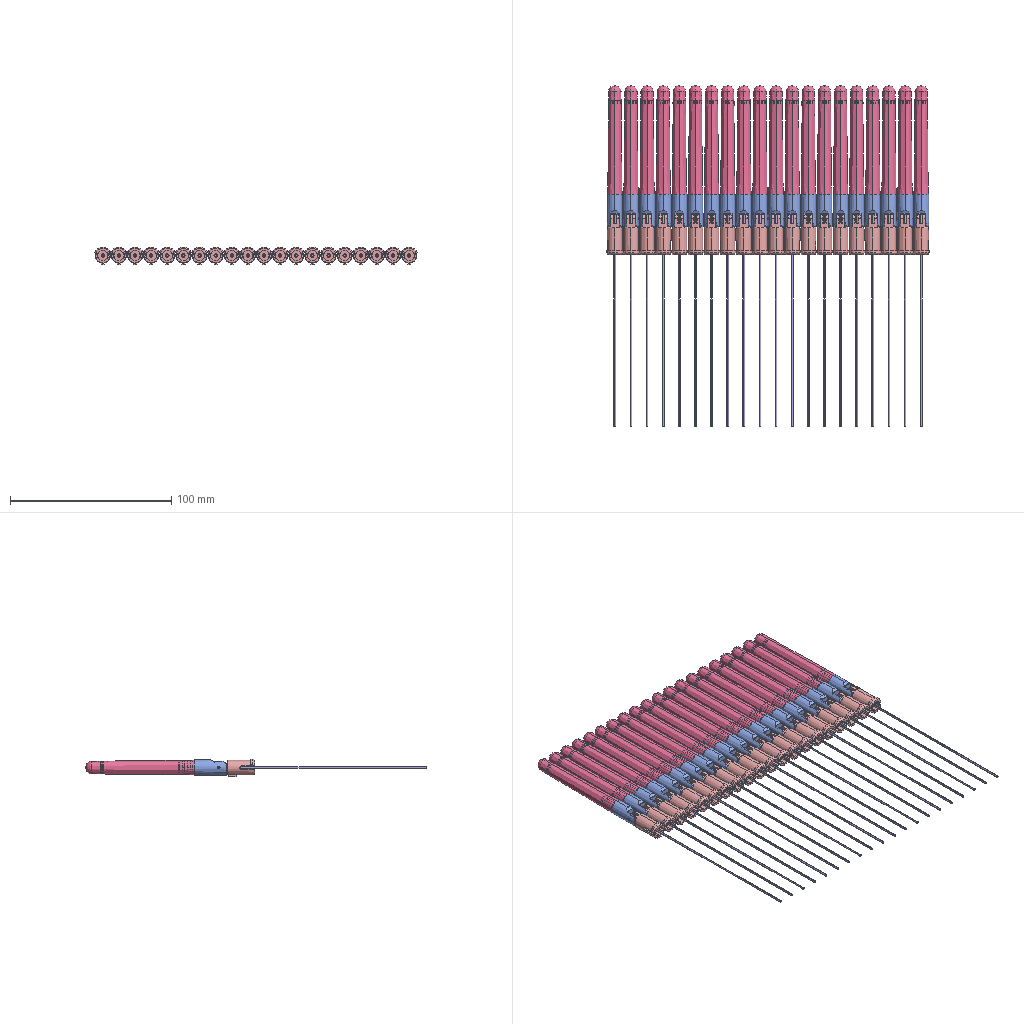Assembly | SolidWorks | 9 different items | 200 placed | box 200 x 211 x 11 mm
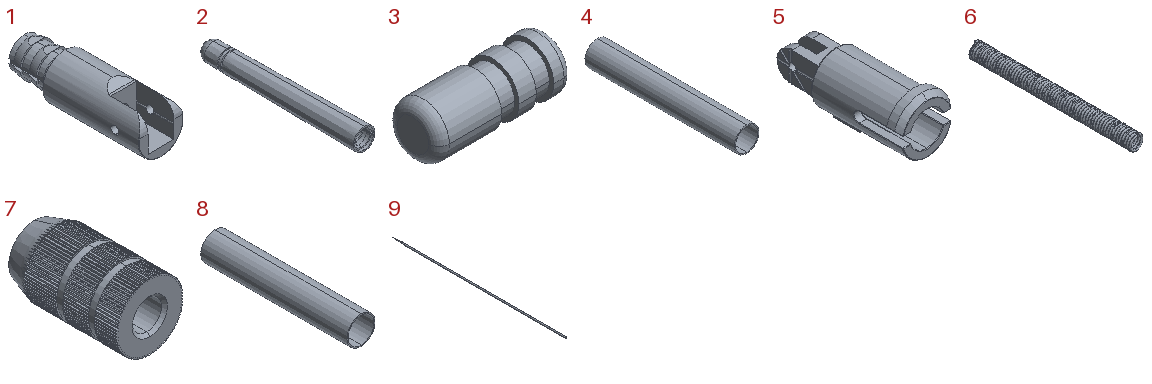Parts list (item | quantity | size | volume | features):
1 | x20 | 9.4 x 28.8 x 9.4 mm | 935.936 mm3 | features ICE 6, Fillet 1, Revolution 1
2 | x20 | 9.2 x 67.3 x 9.2 mm | 2059 mm3 | features ICE 1, Revolution 1
3 | x40 | 3.8 x 1.5 x 1.5 mm | 6.054 mm3 | features Revolution 1
4 | x20 | 4.3 x 26 x 4.3 mm | 66.979 mm3 | features ExtruThin 1
5 | x20 | 10.095 x 25.05 x 11.15 mm | 779.469 mm3 | features ICE 8, Fillet 3, MirrorPattern 1, Revolution 1
6 | x20 | 3.8 x 41.45 x 3.8 mm | 132.538 mm3 | features Helix 1, Sweep 1
7 | x20 | 4.499 x 7.8 x 4.499 mm | 91.087 mm3 | features CirPattern 1, ICE 1, RevCut 1, Revolution 1
8 | x20 | 5 x 26 x 5 mm | 78.414 mm3 | features Extrusion 1
9 | x20 | 1.13 x 143 x 1.13 mm | 137.726 mm3 | features ICE 3, Extrusion 1
Mates (type | each side: item.copy, entity, surface, feature):
Coincident | 5.1 plane | assembly plane | 2 times
Coincident | 5.1 plane | 1.1 plane
Concentric | 5.1 face cylinder Boss-Extrude1 | 1.1 face cylinder Cut-Extrude3
Parallel | 5.1 face plane Revolve1 | 1.1 face plane Revolve1
Coordinate | 5.1 select_type:25 | assembly select_type:11
Concentric | 7.1 face cylinder Revolve1 | 8.1 face cylinder Boss-Extrude1
Coincident | 7.1 face plane Revolve1 | 8.1 face plane Boss-Extrude1
Concentric | 8.1 face cylinder Boss-Extrude1 | 6.1 select_type:24
DistanceDim | 6.1 plane | 7.1 face plane Revolve1
Concentric | 8.1 face cylinder Boss-Extrude1 | 4.1 face cylinder Extrude-Thin1
DistanceDim | 4.1 face plane Extrude-Thin1 | 8.1 face plane Boss-Extrude1
Coincident | 1.1 face plane Cut-Extrude1 | 7.1 face plane Revolve1
Concentric | 1.1 face cylinder Cut-Extrude1 | 8.1 face cylinder Boss-Extrude1
Concentric | 7.1 face cylinder Revolve1 | 9.1 face cylinder Boss-Extrude1
Coincident | 1.1 face plane Cut-Extrude1 | 9.1 face plane Boss-Extrude1
Concentric | 1.1 face cylinder Cut-Extrude3 | 3.1 face cylinder Revolve1
Tangent | 1.1 face cylinder Revolve1 | 3.1 face plane Revolve1
Concentric | 1.1 face cylinder Cut-Extrude3 | 3.2 face cylinder Revolve1
Tangent | 1.1 face cylinder Revolve1 | 3.2 face plane Revolve1
Parallel | 1.1 face plane Cut-Extrude4 | 2.1 face plane Boss-Extrude1
Coincident | 1.1 face plane Revolve1 | 2.1 face plane Revolve1
Concentric | 1.1 edge | 2.1 edge